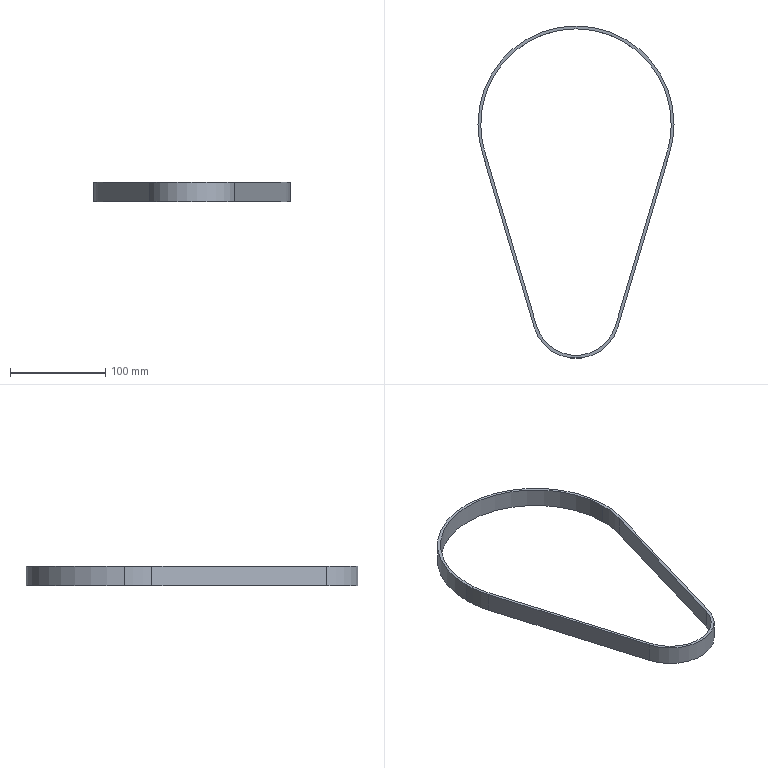Part | SolidWorks | features BaseBody 1 | 1 solid | 14 faces | box 206 x 349.095 x 20 mm | volume 52516 mm3 | cylinder 8 | plane 6 | commonest cylinder face diameters 200 x3 206 x3 86.189 x1 92.189 x1
STEP:
#1=CARTESIAN_POINT('',(103.,0.,-20.));
#2=VERTEX_POINT('',#1);
#3=CARTESIAN_POINT('',(-103.,0.,-20.));
#4=VERTEX_POINT('',#3);
#5=CARTESIAN_POINT('',(0.,0.,-20.));
#6=DIRECTION('',(0.,0.,1.));
#7=DIRECTION('',(1.,0.,0.));
#8=AXIS2_PLACEMENT_3D('',#5,#6,#7);
#9=CIRCLE('',#8,103.);
#10=EDGE_CURVE('',#2,#4,#9,.T.);
#11=ORIENTED_EDGE('',*,*,#10,.T.);
#12=CARTESIAN_POINT('',(-103.,0.,0.));
#13=VERTEX_POINT('',#12);
#14=CARTESIAN_POINT('',(-103.,0.,-20.));
#15=DIRECTION('',(0.,0.,1.));
#16=VECTOR('',#15,1000.);
#17=LINE('',#14,#16);
#18=EDGE_CURVE('',#4,#13,#17,.T.);
#19=ORIENTED_EDGE('',*,*,#18,.T.);
#20=CARTESIAN_POINT('',(103.,0.,0.));
#21=VERTEX_POINT('',#20);
#22=CARTESIAN_POINT('',(0.,0.,0.));
#23=DIRECTION('',(0.,0.,-1.));
#24=DIRECTION('',(1.,0.,0.));
#25=AXIS2_PLACEMENT_3D('',#22,#23,#24);
#26=CIRCLE('',#25,103.);
#27=EDGE_CURVE('',#13,#21,#26,.T.);
#28=ORIENTED_EDGE('',*,*,#27,.T.);
#29=CARTESIAN_POINT('',(103.,0.,-20.));
#30=DIRECTION('',(0.,0.,1.));
#31=VECTOR('',#30,1000.);
#32=LINE('',#29,#31);
#33=EDGE_CURVE('',#2,#21,#32,.T.);
#34=ORIENTED_EDGE('',*,*,#33,.F.);
#35=EDGE_LOOP('',(#11,#19,#28,#34));
#36=FACE_OUTER_BOUND('',#35,.T.);
#37=CARTESIAN_POINT('',(0.,0.,-20.));
#38=DIRECTION('',(0.,0.,1.));
#39=DIRECTION('',(1.,0.,0.));
#40=AXIS2_PLACEMENT_3D('',#37,#38,#39);
#41=CYLINDRICAL_SURFACE('',#40,103.);
#42=ADVANCED_FACE('',(#36),#41,.T.);
#43=CARTESIAN_POINT('',(98.743,-29.306,-20.));
#44=VERTEX_POINT('',#43);
#45=CARTESIAN_POINT('',(0.,0.,-20.));
#46=DIRECTION('',(0.,0.,1.));
#47=DIRECTION('',(1.,0.,0.));
#48=AXIS2_PLACEMENT_3D('',#45,#46,#47);
#49=CIRCLE('',#48,103.);
#50=EDGE_CURVE('',#44,#2,#49,.T.);
#51=ORIENTED_EDGE('',*,*,#50,.T.);
#52=ORIENTED_EDGE('',*,*,#33,.T.);
#53=CARTESIAN_POINT('',(98.743,-29.306,0.));
#54=VERTEX_POINT('',#53);
#55=CARTESIAN_POINT('',(0.,0.,0.));
#56=DIRECTION('',(0.,0.,-1.));
#57=DIRECTION('',(1.,0.,0.));
#58=AXIS2_PLACEMENT_3D('',#55,#56,#57);
#59=CIRCLE('',#58,103.);
#60=EDGE_CURVE('',#21,#54,#59,.T.);
#61=ORIENTED_EDGE('',*,*,#60,.T.);
#62=CARTESIAN_POINT('',(98.743,-29.306,-20.));
#63=DIRECTION('',(0.,0.,-1.));
#64=VECTOR('',#63,1000.);
#65=LINE('',#62,#64);
#66=EDGE_CURVE('',#54,#44,#65,.T.);
#67=ORIENTED_EDGE('',*,*,#66,.T.);
#68=EDGE_LOOP('',(#51,#52,#61,#67));
#69=FACE_OUTER_BOUND('',#68,.T.);
#70=CARTESIAN_POINT('',(0.,0.,-20.));
#71=DIRECTION('',(0.,0.,1.));
#72=DIRECTION('',(1.,0.,0.));
#73=AXIS2_PLACEMENT_3D('',#70,#71,#72);
#74=CYLINDRICAL_SURFACE('',#73,103.);
#75=ADVANCED_FACE('',(#69),#74,.T.);
#76=CARTESIAN_POINT('',(-100.,0.,-20.));
#77=VERTEX_POINT('',#76);
#78=CARTESIAN_POINT('',(-95.867,-28.453,-20.));
#79=VERTEX_POINT('',#78);
#80=CARTESIAN_POINT('',(0.,0.,-20.));
#81=DIRECTION('',(0.,0.,1.));
#82=DIRECTION('',(1.,0.,0.));
#83=AXIS2_PLACEMENT_3D('',#80,#81,#82);
#84=CIRCLE('',#83,100.);
#85=EDGE_CURVE('',#77,#79,#84,.T.);
#86=ORIENTED_EDGE('',*,*,#85,.F.);
#87=CARTESIAN_POINT('',(-100.,0.,0.));
#88=VERTEX_POINT('',#87);
#89=CARTESIAN_POINT('',(-100.,0.,-20.));
#90=DIRECTION('',(0.,0.,1.));
#91=VECTOR('',#90,1000.);
#92=LINE('',#89,#91);
#93=EDGE_CURVE('',#77,#88,#92,.T.);
#94=ORIENTED_EDGE('',*,*,#93,.T.);
#95=CARTESIAN_POINT('',(-95.867,-28.453,0.));
#96=VERTEX_POINT('',#95);
#97=CARTESIAN_POINT('',(0.,0.,0.));
#98=DIRECTION('',(0.,0.,1.));
#99=DIRECTION('',(1.,0.,0.));
#100=AXIS2_PLACEMENT_3D('',#97,#98,#99);
#101=CIRCLE('',#100,100.);
#102=EDGE_CURVE('',#88,#96,#101,.T.);
#103=ORIENTED_EDGE('',*,*,#102,.T.);
#104=CARTESIAN_POINT('',(-95.867,-28.453,-20.));
#105=DIRECTION('',(0.,0.,-1.));
#106=VECTOR('',#105,1000.);
#107=LINE('',#104,#106);
#108=EDGE_CURVE('',#96,#79,#107,.T.);
#109=ORIENTED_EDGE('',*,*,#108,.T.);
#110=EDGE_LOOP('',(#86,#94,#103,#109));
#111=FACE_OUTER_BOUND('',#110,.T.);
#112=CARTESIAN_POINT('',(0.,0.,-20.));
#113=DIRECTION('',(0.,0.,1.));
#114=DIRECTION('',(1.,0.,0.));
#115=AXIS2_PLACEMENT_3D('',#112,#113,#114);
#116=CYLINDRICAL_SURFACE('',#115,100.);
#117=ADVANCED_FACE('',(#111),#116,.F.);
#118=ORIENTED_EDGE('',*,*,#93,.F.);
#119=CARTESIAN_POINT('',(100.,0.,-20.));
#120=VERTEX_POINT('',#119);
#121=CARTESIAN_POINT('',(0.,0.,-20.));
#122=DIRECTION('',(0.,0.,1.));
#123=DIRECTION('',(1.,0.,0.));
#124=AXIS2_PLACEMENT_3D('',#121,#122,#123);
#125=CIRCLE('',#124,100.);
#126=EDGE_CURVE('',#120,#77,#125,.T.);
#127=ORIENTED_EDGE('',*,*,#126,.F.);
#128=CARTESIAN_POINT('',(100.,0.,0.));
#129=VERTEX_POINT('',#128);
#130=CARTESIAN_POINT('',(100.,0.,-20.));
#131=DIRECTION('',(0.,0.,1.));
#132=VECTOR('',#131,1000.);
#133=LINE('',#130,#132);
#134=EDGE_CURVE('',#120,#129,#133,.T.);
#135=ORIENTED_EDGE('',*,*,#134,.T.);
#136=CARTESIAN_POINT('',(0.,0.,0.));
#137=DIRECTION('',(0.,0.,1.));
#138=DIRECTION('',(1.,0.,0.));
#139=AXIS2_PLACEMENT_3D('',#136,#137,#138);
#140=CIRCLE('',#139,100.);
#141=EDGE_CURVE('',#129,#88,#140,.T.);
#142=ORIENTED_EDGE('',*,*,#141,.T.);
#143=EDGE_LOOP('',(#118,#127,#135,#142));
#144=FACE_OUTER_BOUND('',#143,.T.);
#145=CARTESIAN_POINT('',(0.,0.,-20.));
#146=DIRECTION('',(0.,0.,1.));
#147=DIRECTION('',(1.,0.,0.));
#148=AXIS2_PLACEMENT_3D('',#145,#146,#147);
#149=CYLINDRICAL_SURFACE('',#148,100.);
#150=ADVANCED_FACE('',(#144),#149,.F.);
#151=ORIENTED_EDGE('',*,*,#18,.F.);
#152=CARTESIAN_POINT('',(-98.743,-29.306,-20.));
#153=VERTEX_POINT('',#152);
#154=CARTESIAN_POINT('',(0.,0.,-20.));
#155=DIRECTION('',(0.,0.,1.));
#156=DIRECTION('',(1.,0.,0.));
#157=AXIS2_PLACEMENT_3D('',#154,#155,#156);
#158=CIRCLE('',#157,103.);
#159=EDGE_CURVE('',#4,#153,#158,.T.);
#160=ORIENTED_EDGE('',*,*,#159,.T.);
#161=CARTESIAN_POINT('',(-98.743,-29.306,0.));
#162=VERTEX_POINT('',#161);
#163=CARTESIAN_POINT('',(-98.743,-29.306,-20.));
#164=DIRECTION('',(0.,0.,1.));
#165=VECTOR('',#164,1000.);
#166=LINE('',#163,#165);
#167=EDGE_CURVE('',#153,#162,#166,.T.);
#168=ORIENTED_EDGE('',*,*,#167,.T.);
#169=CARTESIAN_POINT('',(0.,0.,0.));
#170=DIRECTION('',(0.,0.,-1.));
#171=DIRECTION('',(1.,0.,0.));
#172=AXIS2_PLACEMENT_3D('',#169,#170,#171);
#173=CIRCLE('',#172,103.);
#174=EDGE_CURVE('',#162,#13,#173,.T.);
#175=ORIENTED_EDGE('',*,*,#174,.T.);
#176=EDGE_LOOP('',(#151,#160,#168,#175));
#177=FACE_OUTER_BOUND('',#176,.T.);
#178=CARTESIAN_POINT('',(0.,0.,-20.));
#179=DIRECTION('',(0.,0.,1.));
#180=DIRECTION('',(1.,0.,0.));
#181=AXIS2_PLACEMENT_3D('',#178,#179,#180);
#182=CYLINDRICAL_SURFACE('',#181,103.);
#183=ADVANCED_FACE('',(#177),#182,.T.);
#184=ORIENTED_EDGE('',*,*,#174,.F.);
#185=CARTESIAN_POINT('',(-44.19,-213.115,0.));
#186=VERTEX_POINT('',#185);
#187=CARTESIAN_POINT('',(-44.19,-213.115,0.));
#188=DIRECTION('',(-0.2845,0.9587,0.));
#189=VECTOR('',#188,1000.);
#190=LINE('',#187,#189);
#191=EDGE_CURVE('',#186,#162,#190,.T.);
#192=ORIENTED_EDGE('',*,*,#191,.F.);
#193=CARTESIAN_POINT('',(44.19,-213.115,0.));
#194=VERTEX_POINT('',#193);
#195=CARTESIAN_POINT('',(0.,-200.,0.));
#196=DIRECTION('',(0.,0.,-1.));
#197=DIRECTION('',(1.,0.,0.));
#198=AXIS2_PLACEMENT_3D('',#195,#196,#197);
#199=CIRCLE('',#198,46.095);
#200=EDGE_CURVE('',#194,#186,#199,.T.);
#201=ORIENTED_EDGE('',*,*,#200,.F.);
#202=CARTESIAN_POINT('',(98.743,-29.306,0.));
#203=DIRECTION('',(-0.2845,-0.9587,0.));
#204=VECTOR('',#203,1000.);
#205=LINE('',#202,#204);
#206=EDGE_CURVE('',#54,#194,#205,.T.);
#207=ORIENTED_EDGE('',*,*,#206,.F.);
#208=ORIENTED_EDGE('',*,*,#60,.F.);
#209=ORIENTED_EDGE('',*,*,#27,.F.);
#210=EDGE_LOOP('',(#184,#192,#201,#207,#208,#209));
#211=FACE_OUTER_BOUND('',#210,.T.);
#212=CARTESIAN_POINT('',(95.867,-28.453,0.));
#213=VERTEX_POINT('',#212);
#214=CARTESIAN_POINT('',(0.,0.,0.));
#215=DIRECTION('',(0.,0.,1.));
#216=DIRECTION('',(1.,0.,0.));
#217=AXIS2_PLACEMENT_3D('',#214,#215,#216);
#218=CIRCLE('',#217,100.);
#219=EDGE_CURVE('',#213,#129,#218,.T.);
#220=ORIENTED_EDGE('',*,*,#219,.F.);
#221=CARTESIAN_POINT('',(41.314,-212.262,0.));
#222=VERTEX_POINT('',#221);
#223=CARTESIAN_POINT('',(41.314,-212.262,0.));
#224=DIRECTION('',(0.2845,0.9587,0.));
#225=VECTOR('',#224,1000.);
#226=LINE('',#223,#225);
#227=EDGE_CURVE('',#222,#213,#226,.T.);
#228=ORIENTED_EDGE('',*,*,#227,.F.);
#229=CARTESIAN_POINT('',(-41.314,-212.262,0.));
#230=VERTEX_POINT('',#229);
#231=CARTESIAN_POINT('',(0.,-200.,0.));
#232=DIRECTION('',(0.,0.,1.));
#233=DIRECTION('',(1.,0.,0.));
#234=AXIS2_PLACEMENT_3D('',#231,#232,#233);
#235=CIRCLE('',#234,43.095);
#236=EDGE_CURVE('',#230,#222,#235,.T.);
#237=ORIENTED_EDGE('',*,*,#236,.F.);
#238=CARTESIAN_POINT('',(-95.867,-28.453,0.));
#239=DIRECTION('',(0.2845,-0.9587,0.));
#240=VECTOR('',#239,1000.);
#241=LINE('',#238,#240);
#242=EDGE_CURVE('',#96,#230,#241,.T.);
#243=ORIENTED_EDGE('',*,*,#242,.F.);
#244=ORIENTED_EDGE('',*,*,#102,.F.);
#245=ORIENTED_EDGE('',*,*,#141,.F.);
#246=EDGE_LOOP('',(#220,#228,#237,#243,#244,#245));
#247=FACE_BOUND('',#246,.T.);
#248=CARTESIAN_POINT('',(0.,0.,0.));
#249=DIRECTION('',(0.,0.,-1.));
#250=DIRECTION('',(-1.,0.,0.));
#251=AXIS2_PLACEMENT_3D('',#248,#249,#250);
#252=PLANE('',#251);
#253=ADVANCED_FACE('',(#211,#247),#252,.F.);
#254=CARTESIAN_POINT('',(-44.19,-213.115,-20.));
#255=VERTEX_POINT('',#254);
#256=CARTESIAN_POINT('',(-44.19,-213.115,-20.));
#257=DIRECTION('',(-0.2845,0.9587,0.));
#258=VECTOR('',#257,1000.);
#259=LINE('',#256,#258);
#260=EDGE_CURVE('',#255,#153,#259,.T.);
#261=ORIENTED_EDGE('',*,*,#260,.T.);
#262=ORIENTED_EDGE('',*,*,#159,.F.);
#263=ORIENTED_EDGE('',*,*,#10,.F.);
#264=ORIENTED_EDGE('',*,*,#50,.F.);
#265=CARTESIAN_POINT('',(44.19,-213.115,-20.));
#266=VERTEX_POINT('',#265);
#267=CARTESIAN_POINT('',(98.743,-29.306,-20.));
#268=DIRECTION('',(-0.2845,-0.9587,0.));
#269=VECTOR('',#268,1000.);
#270=LINE('',#267,#269);
#271=EDGE_CURVE('',#44,#266,#270,.T.);
#272=ORIENTED_EDGE('',*,*,#271,.T.);
#273=CARTESIAN_POINT('',(0.,-200.,-20.));
#274=DIRECTION('',(0.,0.,-1.));
#275=DIRECTION('',(1.,0.,0.));
#276=AXIS2_PLACEMENT_3D('',#273,#274,#275);
#277=CIRCLE('',#276,46.095);
#278=EDGE_CURVE('',#266,#255,#277,.T.);
#279=ORIENTED_EDGE('',*,*,#278,.T.);
#280=EDGE_LOOP('',(#261,#262,#263,#264,#272,#279));
#281=FACE_OUTER_BOUND('',#280,.T.);
#282=CARTESIAN_POINT('',(-41.314,-212.262,-20.));
#283=VERTEX_POINT('',#282);
#284=CARTESIAN_POINT('',(41.314,-212.262,-20.));
#285=VERTEX_POINT('',#284);
#286=CARTESIAN_POINT('',(0.,-200.,-20.));
#287=DIRECTION('',(0.,0.,1.));
#288=DIRECTION('',(1.,0.,0.));
#289=AXIS2_PLACEMENT_3D('',#286,#287,#288);
#290=CIRCLE('',#289,43.095);
#291=EDGE_CURVE('',#283,#285,#290,.T.);
#292=ORIENTED_EDGE('',*,*,#291,.T.);
#293=CARTESIAN_POINT('',(95.867,-28.453,-20.));
#294=VERTEX_POINT('',#293);
#295=CARTESIAN_POINT('',(41.314,-212.262,-20.));
#296=DIRECTION('',(0.2845,0.9587,0.));
#297=VECTOR('',#296,1000.);
#298=LINE('',#295,#297);
#299=EDGE_CURVE('',#285,#294,#298,.T.);
#300=ORIENTED_EDGE('',*,*,#299,.T.);
#301=CARTESIAN_POINT('',(0.,0.,-20.));
#302=DIRECTION('',(0.,0.,1.));
#303=DIRECTION('',(1.,0.,0.));
#304=AXIS2_PLACEMENT_3D('',#301,#302,#303);
#305=CIRCLE('',#304,100.);
#306=EDGE_CURVE('',#294,#120,#305,.T.);
#307=ORIENTED_EDGE('',*,*,#306,.T.);
#308=ORIENTED_EDGE('',*,*,#126,.T.);
#309=ORIENTED_EDGE('',*,*,#85,.T.);
#310=CARTESIAN_POINT('',(-95.867,-28.453,-20.));
#311=DIRECTION('',(0.2845,-0.9587,0.));
#312=VECTOR('',#311,1000.);
#313=LINE('',#310,#312);
#314=EDGE_CURVE('',#79,#283,#313,.T.);
#315=ORIENTED_EDGE('',*,*,#314,.T.);
#316=EDGE_LOOP('',(#292,#300,#307,#308,#309,#315));
#317=FACE_BOUND('',#316,.T.);
#318=CARTESIAN_POINT('',(0.,0.,-20.));
#319=DIRECTION('',(0.,0.,-1.));
#320=DIRECTION('',(-1.,0.,0.));
#321=AXIS2_PLACEMENT_3D('',#318,#319,#320);
#322=PLANE('',#321);
#323=ADVANCED_FACE('',(#281,#317),#322,.T.);
#324=ORIENTED_EDGE('',*,*,#271,.F.);
#325=ORIENTED_EDGE('',*,*,#66,.F.);
#326=ORIENTED_EDGE('',*,*,#206,.T.);
#327=CARTESIAN_POINT('',(44.19,-213.115,-20.));
#328=DIRECTION('',(0.,0.,-1.));
#329=VECTOR('',#328,1000.);
#330=LINE('',#327,#329);
#331=EDGE_CURVE('',#194,#266,#330,.T.);
#332=ORIENTED_EDGE('',*,*,#331,.T.);
#333=EDGE_LOOP('',(#324,#325,#326,#332));
#334=FACE_OUTER_BOUND('',#333,.T.);
#335=CARTESIAN_POINT('',(98.743,-29.306,-20.));
#336=DIRECTION('',(0.9587,-0.2845,0.));
#337=DIRECTION('',(0.2845,0.9587,0.));
#338=AXIS2_PLACEMENT_3D('',#335,#336,#337);
#339=PLANE('',#338);
#340=ADVANCED_FACE('',(#334),#339,.T.);
#341=ORIENTED_EDGE('',*,*,#260,.F.);
#342=CARTESIAN_POINT('',(-44.19,-213.115,-20.));
#343=DIRECTION('',(0.,0.,1.));
#344=VECTOR('',#343,1000.);
#345=LINE('',#342,#344);
#346=EDGE_CURVE('',#255,#186,#345,.T.);
#347=ORIENTED_EDGE('',*,*,#346,.T.);
#348=ORIENTED_EDGE('',*,*,#191,.T.);
#349=ORIENTED_EDGE('',*,*,#167,.F.);
#350=EDGE_LOOP('',(#341,#347,#348,#349));
#351=FACE_OUTER_BOUND('',#350,.T.);
#352=CARTESIAN_POINT('',(-98.743,-29.306,-20.));
#353=DIRECTION('',(-0.9587,-0.2845,0.));
#354=DIRECTION('',(0.2845,-0.9587,0.));
#355=AXIS2_PLACEMENT_3D('',#352,#353,#354);
#356=PLANE('',#355);
#357=ADVANCED_FACE('',(#351),#356,.T.);
#358=ORIENTED_EDGE('',*,*,#278,.F.);
#359=ORIENTED_EDGE('',*,*,#331,.F.);
#360=ORIENTED_EDGE('',*,*,#200,.T.);
#361=ORIENTED_EDGE('',*,*,#346,.F.);
#362=EDGE_LOOP('',(#358,#359,#360,#361));
#363=FACE_OUTER_BOUND('',#362,.T.);
#364=CARTESIAN_POINT('',(0.,-200.,-20.));
#365=DIRECTION('',(0.,0.,1.));
#366=DIRECTION('',(1.,0.,0.));
#367=AXIS2_PLACEMENT_3D('',#364,#365,#366);
#368=CYLINDRICAL_SURFACE('',#367,46.095);
#369=ADVANCED_FACE('',(#363),#368,.T.);
#370=CARTESIAN_POINT('',(-41.314,-212.262,-20.));
#371=DIRECTION('',(0.,0.,1.));
#372=VECTOR('',#371,1000.);
#373=LINE('',#370,#372);
#374=EDGE_CURVE('',#283,#230,#373,.T.);
#375=ORIENTED_EDGE('',*,*,#374,.F.);
#376=ORIENTED_EDGE('',*,*,#314,.F.);
#377=ORIENTED_EDGE('',*,*,#108,.F.);
#378=ORIENTED_EDGE('',*,*,#242,.T.);
#379=EDGE_LOOP('',(#375,#376,#377,#378));
#380=FACE_OUTER_BOUND('',#379,.T.);
#381=CARTESIAN_POINT('',(-41.314,-212.262,-20.));
#382=DIRECTION('',(-0.9587,-0.2845,0.));
#383=DIRECTION('',(0.2845,-0.9587,0.));
#384=AXIS2_PLACEMENT_3D('',#381,#382,#383);
#385=PLANE('',#384);
#386=ADVANCED_FACE('',(#380),#385,.F.);
#387=ORIENTED_EDGE('',*,*,#134,.F.);
#388=ORIENTED_EDGE('',*,*,#306,.F.);
#389=CARTESIAN_POINT('',(95.867,-28.453,-20.));
#390=DIRECTION('',(0.,0.,-1.));
#391=VECTOR('',#390,1000.);
#392=LINE('',#389,#391);
#393=EDGE_CURVE('',#213,#294,#392,.T.);
#394=ORIENTED_EDGE('',*,*,#393,.F.);
#395=ORIENTED_EDGE('',*,*,#219,.T.);
#396=EDGE_LOOP('',(#387,#388,#394,#395));
#397=FACE_OUTER_BOUND('',#396,.T.);
#398=CARTESIAN_POINT('',(0.,0.,-20.));
#399=DIRECTION('',(0.,0.,1.));
#400=DIRECTION('',(1.,0.,0.));
#401=AXIS2_PLACEMENT_3D('',#398,#399,#400);
#402=CYLINDRICAL_SURFACE('',#401,100.);
#403=ADVANCED_FACE('',(#397),#402,.F.);
#404=ORIENTED_EDGE('',*,*,#393,.T.);
#405=ORIENTED_EDGE('',*,*,#299,.F.);
#406=CARTESIAN_POINT('',(41.314,-212.262,-20.));
#407=DIRECTION('',(0.,0.,-1.));
#408=VECTOR('',#407,1000.);
#409=LINE('',#406,#408);
#410=EDGE_CURVE('',#222,#285,#409,.T.);
#411=ORIENTED_EDGE('',*,*,#410,.F.);
#412=ORIENTED_EDGE('',*,*,#227,.T.);
#413=EDGE_LOOP('',(#404,#405,#411,#412));
#414=FACE_OUTER_BOUND('',#413,.T.);
#415=CARTESIAN_POINT('',(95.867,-28.453,-20.));
#416=DIRECTION('',(0.9587,-0.2845,0.));
#417=DIRECTION('',(0.2845,0.9587,0.));
#418=AXIS2_PLACEMENT_3D('',#415,#416,#417);
#419=PLANE('',#418);
#420=ADVANCED_FACE('',(#414),#419,.F.);
#421=ORIENTED_EDGE('',*,*,#410,.T.);
#422=ORIENTED_EDGE('',*,*,#291,.F.);
#423=ORIENTED_EDGE('',*,*,#374,.T.);
#424=ORIENTED_EDGE('',*,*,#236,.T.);
#425=EDGE_LOOP('',(#421,#422,#423,#424));
#426=FACE_OUTER_BOUND('',#425,.T.);
#427=CARTESIAN_POINT('',(0.,-200.,-20.));
#428=DIRECTION('',(0.,0.,1.));
#429=DIRECTION('',(1.,0.,0.));
#430=AXIS2_PLACEMENT_3D('',#427,#428,#429);
#431=CYLINDRICAL_SURFACE('',#430,43.095);
#432=ADVANCED_FACE('',(#426),#431,.F.);
#433=CLOSED_SHELL('',(#42,#75,#117,#150,#183,#253,#323,#340,#357,#369,#386,#403,#420,#432));
#434=MANIFOLD_SOLID_BREP('',#433);
#435=CARTESIAN_POINT('',(0.,0.,0.));
#436=DIRECTION('',(0.,0.,1.));
#437=DIRECTION('',(1.,0.,0.));
#438=AXIS2_PLACEMENT_3D('',#435,#436,#437);
#439=(LENGTH_UNIT()NAMED_UNIT(*)SI_UNIT(.MILLI.,.METRE.));
#440=UNCERTAINTY_MEASURE_WITH_UNIT(LENGTH_MEASURE(0.00001),#439,'','');
#441=(NAMED_UNIT(*)PLANE_ANGLE_UNIT()SI_UNIT($,.RADIAN.));
#442=(NAMED_UNIT(*)SI_UNIT($,.STERADIAN.)SOLID_ANGLE_UNIT());
#443=(GEOMETRIC_REPRESENTATION_CONTEXT(3)GLOBAL_UNCERTAINTY_ASSIGNED_CONTEXT((#440))GLOBAL_UNIT_ASSIGNED_CONTEXT((#439,#441,#442))REPRESENTATION_CONTEXT('',''));
#444=ADVANCED_BREP_SHAPE_REPRESENTATION('',(#434,#438),#443);